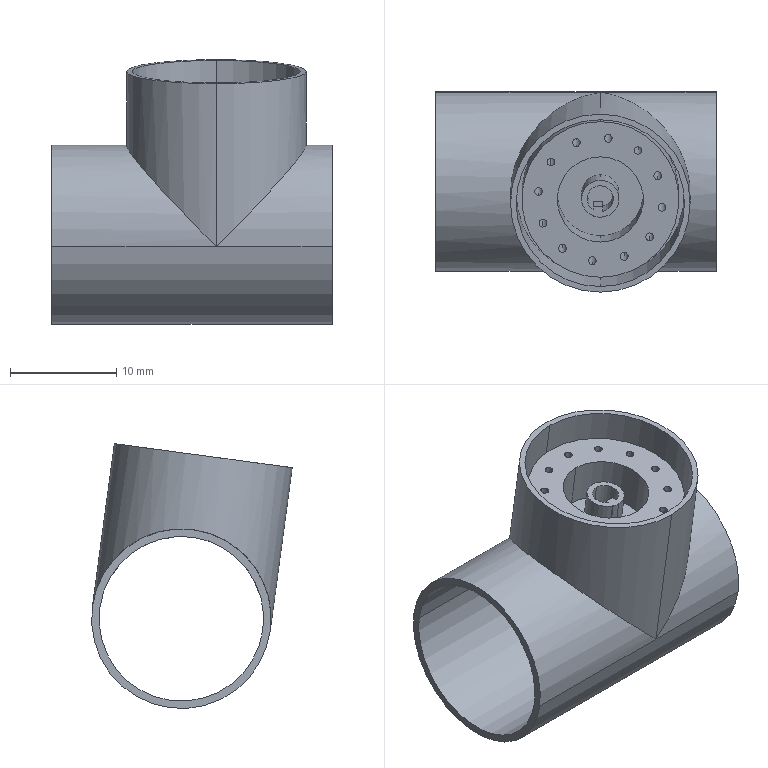Part | SolidWorks | features SplitBody 1 | 1 solid | 55 faces | box 26.4 x 18.89 x 24.926 mm | volume 1940 mm3 | cylinder 42 | plane 13 | commonest cylinder face diameters 0.739 x24 16.896 x5 3.52 x3 2.464 x2 8.096 x2 14.784 x2